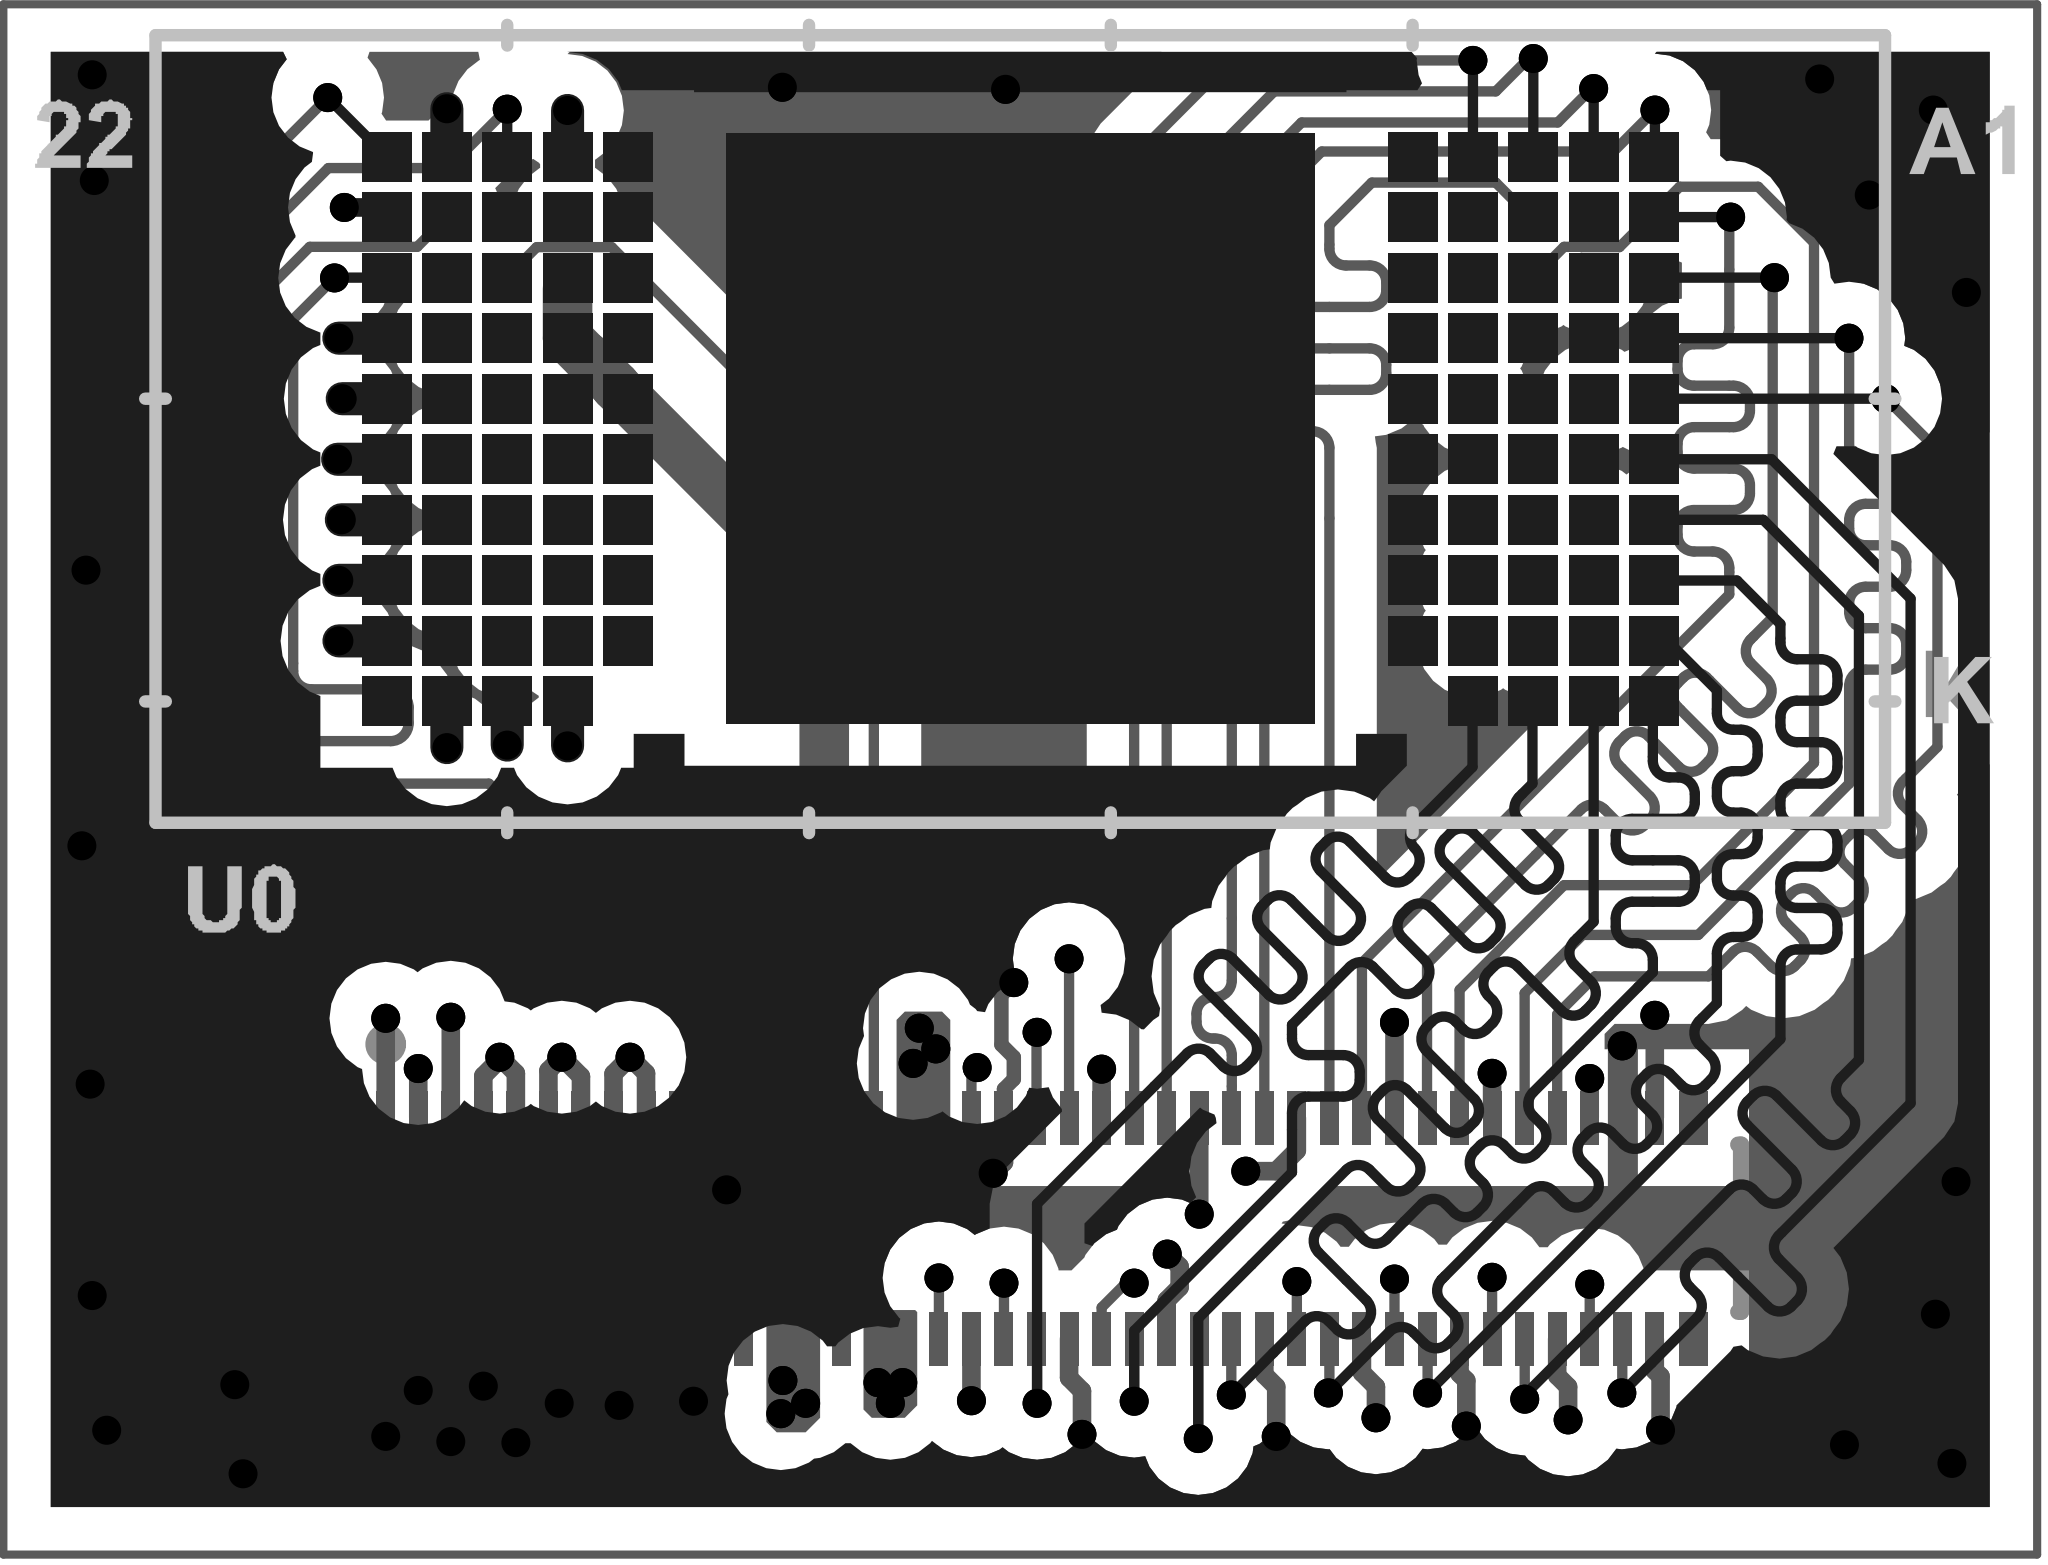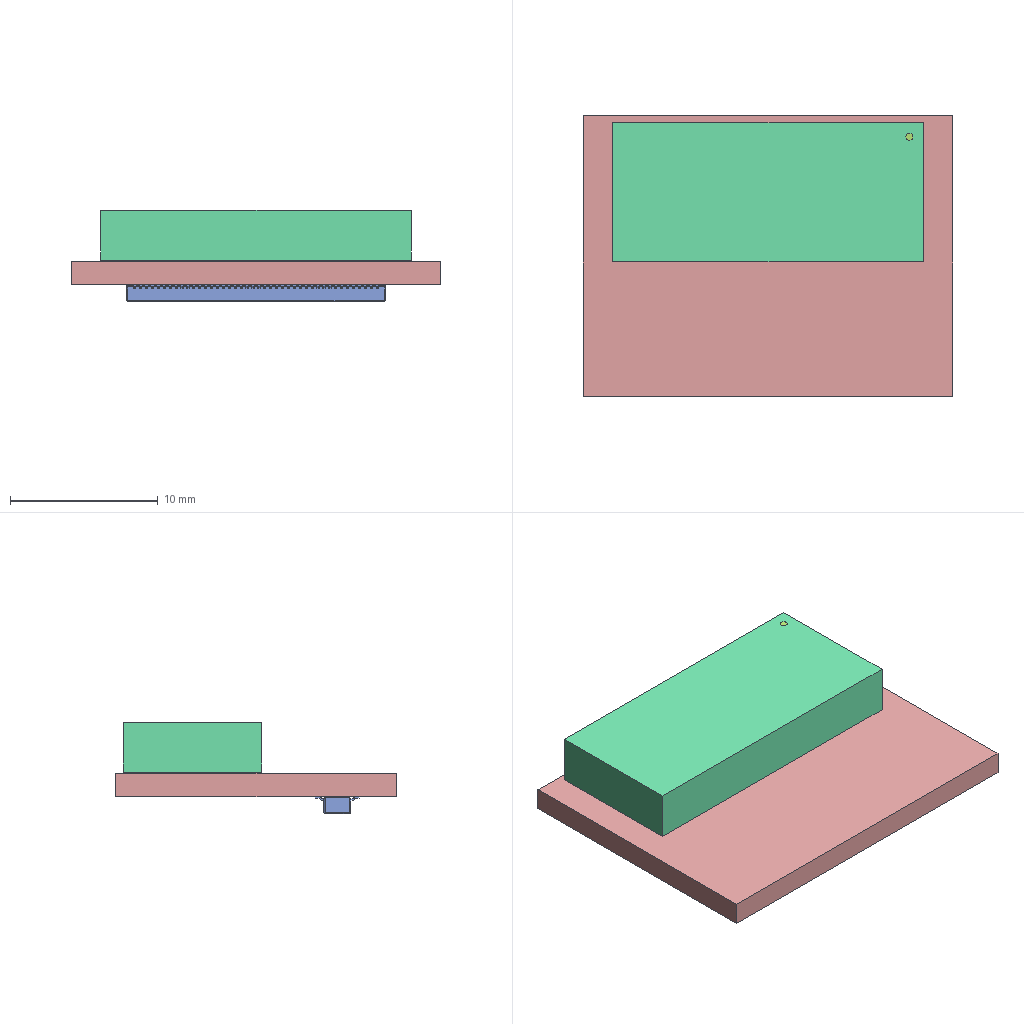Circuit board layout | Altium Designer | box 25 x 19 x 6.2 mm
Layer stack:
# Altium Designer layer stack of  (unit mm; dielectric type: 0 none, 1 core, 2 prepreg, 3 surface material)
index,name,kind,layer,copper_thickness_mm,dielectric_type,dielectric_thickness_mm,dielectric_material,dielectric_constant
0,Top Paste,other,,,,,,
1,Top Overlay,other,,,,,,
2,Top Solder,dielectric,,,3,0.0102,Solder Resist,3.5
3,Top Layer,copper,Top Layer,0.035,,,,
4,Dielectric1,dielectric,,,1,0.0711,PP-006,4.1
5,GND,copper,GND,0.0356,,,,
6,Dielectric8,dielectric,,,2,0.32,FR-4,4.8
7,SIG3,copper,SIG3,0.0356,,,,
8,Dielectric2,dielectric,,,1,0.32,FR-4,4.8
9,POWER4,copper,POWER4,0.0356,,,,
10,Dielectric6,dielectric,,,2,0.32,FR-4,4.8
11,GND5,copper,GND5,0.0356,,,,
12,Dielectric7,dielectric,,,1,0.32,FR-4,4.8
13,Bottom Layer,copper,Bottom Layer,0.035,,,,
14,Bottom Solder,dielectric,,,3,0.0102,Solder Resist,3.5
15,Bottom Overlay,other,,,,,,
16,Bottom Paste,other,,,,,,
# drill layer pairs: low layer,high layer
drill_pair,Top Layer,Bottom Layer
Part placement:
Designator,Comment,Layer,Footprint,Center-X(mm),Center-Y(mm),Rotation
J0,DF40C-80DP-0.4V_51,BottomLayer,HIROSE_DF40C-80DP-0.4V_51_0,12.5,4,360
U0,DLP4500AFQD,TopLayer,LGA_0AFQD_TEX,12.5,13.795,180
Pad and via stacks:
# Altium Designer via and pad stacks of  (unit mm). Each distinct definition once, with the count of objects using it.
# via: kind,start_layer,end_layer,hole_mm,diameter_mm,mode(0 simple;1 top-mid-bottom;2 full stack),diameter_per_layer,count,example_net
# pad: kind,layer,hole_mm,hole_type(0 round;1 square;2 slot),plating,top_size,top_shape(1 round;2 rect;3 octagon;9 rounded rect),mid_size,bottom_size,mode,footprint,size_per_layer,count,example
pad,Bottom Layer,0,0,plated,0.23x0.66,2,0.23x0.66,0.23x0.66,0,HIROSE_DF40C-80DP-0.4V_51_0,,80,J0.1
pad,Bottom Layer,0,0,plated,0.35x0.66,2,0.35x0.66,0.35x0.66,0,HIROSE_DF40C-80DP-0.4V_51_0,,4,J0.81
pad,Top Layer,0,0,plated,7.239x7.239,2,7.239x7.239,7.239x7.239,0,LGA_0AFQD_TEX,,1,U0.99
pad,Top Layer,0,0,plated,0.6096x0.6096,2,0.6096x0.6096,0.6096x0.6096,0,LGA_0AFQD_TEX,,98,U0.A22
via,Top Layer,Bottom Layer,0.2032,0.3556,0,,150,GND
Copper pours:
name,layer,net,type(0 solid;1 hatched;2 none)
Bottom Layer-No Net,Bottom Layer,GND,0
Bottom Layer-No Net,Bottom Layer,VOFFSET,0
Bottom Layer-No Net,Bottom Layer,VRST,0
Bottom Layer-No Net,Bottom Layer,VREF,0
Bottom Layer-No Net,SIG3,GND,0
Bottom Layer-No Net,SIG3,VOFFSET,0
Bottom Layer-No Net,SIG3,VRST,0
Bottom Layer-No Net,SIG3,VREF,0
Bottom Layer-No Net,Top Layer,GND,0
Design rules, without the lines most boards share:
# Altium Designer design rules of  (exported by Altium Designer, unit mm)
# columns: name | kind | enabled | priority | scope1 | scope2 | descriptor | typed fields (field=value)
Clearance_1 | 0 | enabled | 1 | inpolygon | All | Clearance Constraint (Gap=5mil) (inpolygon),(All) | gap=0.127
Clearance | 0 | enabled | 2 | All | All | Clearance Constraint (Gap=5mil) (All),(All) | gap=0.127
Width | 2 | enabled | 1 | All | All | Width Constraint (Min=5mil) (Max=40mil) (Preferred=5mil) (All) |
PlaneConnect | 6 | enabled | 1 | All | All | Power Plane Connect Rule(Direct Connect )(Expansion=20mil) (Conductor Width=10mil) (Air Gap=10mil) (Entries=4) (All) | relief_conductor_width=0.254 relief_entries=4 relief_expansion=0.508
RoutingCorners | 10 | enabled | 1 | All | All | Routing Corners (Style=Round) (Min Setback=100mil) (Max Setback=100mil) (All) |
RoutingVias | 11 | enabled | 1 | All | All | Routing Via (MinHoleWidth=8mil) (MaxHoleWidth=8mil) (PreferredHoleWidth=8mil) (MinWidth=14mil) (MaxWidth=14mil) (PreferedWidth=14mil) (All) | via_min_hole=0.2032 via_max_hole=0.2032 via_preferred_diameter=0.3556 via_preferred_hole=0.2032
PlaneClearance | 12 | enabled | 1 | All | All | Power Plane Clearance (Clearance =5mil) (All) | clearance=0.127
SolderMaskExpansion | 13 | enabled | 1 | All | All | Solder Mask Expansion (Expansion =4mil) (All) | expansion=0.1016
PolygonConnect | 20 | enabled | 1 | All | All | Polygon Connect Rule(Direct Connect )(Conductor Width=10mil) (Relief Angle=90 Angle) (Entries=4) (Air Gap Width=10mil) (All),(All) | connect_style(0=relief,1=direct,2=none)=1 relief_conductor_width=0.254 relief_entries=4
HoleSize | 42 | enabled | 1 | All | All | Hole Size Constraint (Min=1mil) (Max=196.85mil) (All) |
DiffPairsRouting | 51 | enabled | 1 | All | All | Differential Pairs Uncoupled Length using the Gap Constraints (Min=5mil) (Max=5mil) (Prefered=5mil)  and Width Constraints (Min=15mil) (Max=15mil) (Prefered=15mil) (All) |
HoleToHoleClearance | 52 | enabled | 1 | All | All | Hole To Hole Clearance (Gap=0mil) (All),(All) | gap=0
MinimumSolderMaskSliver | 53 | enabled | 1 | All | All | Minimum Solder Mask Sliver (Gap=0mil) (All),(All) |
SilkToSolderMaskClearance | 54 | enabled | 1 | IsPad | All | Silk To Solder Mask (Clearance=0mil) (IsPad),(All) |
SilkToSilkClearance | 55 | enabled | 1 | All | All | Silk to Silk (Clearance=0mil) (All),(All) |
Classes set for this board:
# Altium Designer classes of  (member kind: 0 net, 1 component, 2 from-to, 3 pad, 4 layer, 5 differential pair, 6 design channel, 7 polygon, 8 structure, 9 xSignal)
# columns: class name | member kind | superclass | members
DLP4500 | 1 | no | J0; U0;